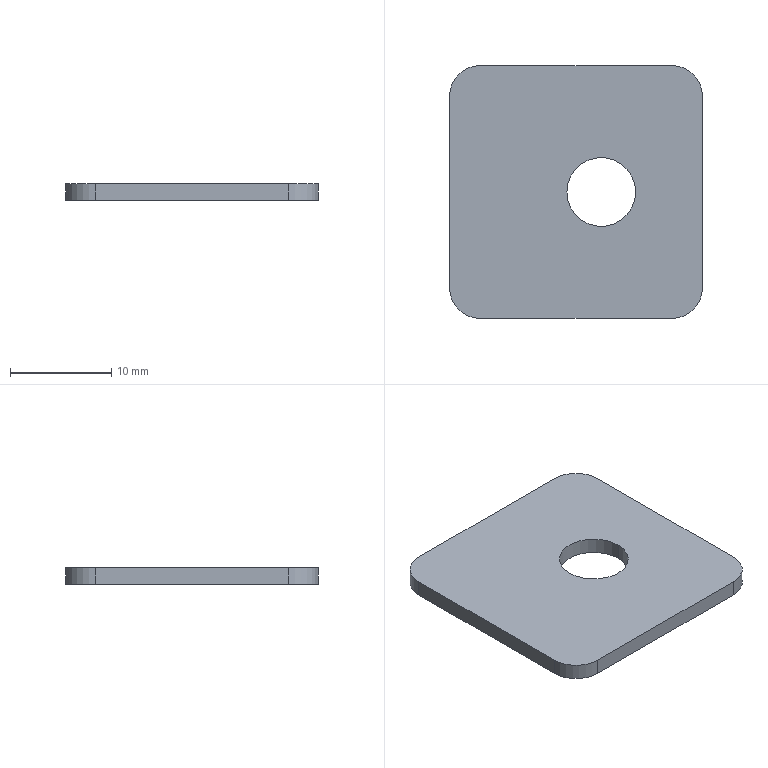Part | STEP file | J454-EBZ05-33-03-Part-1-2 | 1 solid | 12 faces | box 25 x 25 x 1.6 mm | volume 929.532 mm3 | cylinder 6 | plane 6 | commonest cylinder face diameters 6 x4 6.8 x2
STEP:
#1=CARTESIAN_POINT('',(0.,0.,0.));
#2=DIRECTION('',(0.,0.,1.));
#3=DIRECTION('',(1.,0.,0.));
#4=AXIS2_PLACEMENT_3D('',#1,#2,#3);
#5=CARTESIAN_POINT('',(11.6,12.5,0.));
#6=VERTEX_POINT('',#5);
#7=CARTESIAN_POINT('',(11.6,12.5,-1.6));
#8=VERTEX_POINT('',#7);
#9=CARTESIAN_POINT('',(11.6,12.5,0.));
#10=DIRECTION('',(0.,0.,-1.));
#11=VECTOR('',#10,1.);
#12=LINE('',#9,#11);
#13=CARTESIAN_POINT('',(15.,12.5,0.));
#14=DIRECTION('',(0.,0.,-1.));
#15=DIRECTION('',(-1.,0.,0.));
#16=AXIS2_PLACEMENT_3D('',#13,#14,#15);
#17=CYLINDRICAL_SURFACE('',#16,3.4);
#18=CARTESIAN_POINT('',(6.283,0.));
#19=DIRECTION('',(0.,1.));
#20=VECTOR('',#19,1.);
#21=LINE('',#18,#20);
#22=(GEOMETRIC_REPRESENTATION_CONTEXT(2)PARAMETRIC_REPRESENTATION_CONTEXT()REPRESENTATION_CONTEXT('',''));
#23=DEFINITIONAL_REPRESENTATION('',(#21),#22);
#24=PCURVE('',#17,#23);
#25=CARTESIAN_POINT('',(15.,12.5,0.));
#26=DIRECTION('',(0.,0.,-1.));
#27=DIRECTION('',(-1.,0.,0.));
#28=AXIS2_PLACEMENT_3D('',#25,#26,#27);
#29=CYLINDRICAL_SURFACE('',#28,3.4);
#30=CARTESIAN_POINT('',(0.,0.));
#31=DIRECTION('',(0.,1.));
#32=VECTOR('',#31,1.);
#33=LINE('',#30,#32);
#34=(GEOMETRIC_REPRESENTATION_CONTEXT(2)PARAMETRIC_REPRESENTATION_CONTEXT()REPRESENTATION_CONTEXT('',''));
#35=DEFINITIONAL_REPRESENTATION('',(#33),#34);
#36=PCURVE('',#29,#35);
#37=SURFACE_CURVE('',#12,(#24,#36),.PCURVE_S1.);
#38=EDGE_CURVE('',#6,#8,#37,.T.);
#39=ORIENTED_EDGE('',*,*,#38,.T.);
#40=CARTESIAN_POINT('',(18.4,12.5,-1.6));
#41=VERTEX_POINT('',#40);
#42=CARTESIAN_POINT('',(15.,12.5,-1.6));
#43=DIRECTION('',(0.,0.,1.));
#44=DIRECTION('',(1.,0.,0.));
#45=AXIS2_PLACEMENT_3D('',#42,#43,#44);
#46=CIRCLE('',#45,3.4);
#47=CARTESIAN_POINT('',(9.425,1.6));
#48=DIRECTION('',(-1.,0.));
#49=VECTOR('',#48,1.);
#50=LINE('',#47,#49);
#51=(GEOMETRIC_REPRESENTATION_CONTEXT(2)PARAMETRIC_REPRESENTATION_CONTEXT()REPRESENTATION_CONTEXT('',''));
#52=DEFINITIONAL_REPRESENTATION('',(#50),#51);
#53=PCURVE('',#17,#52);
#54=CARTESIAN_POINT('',(12.5,12.5,-1.6));
#55=DIRECTION('',(0.,0.,-1.));
#56=DIRECTION('',(-1.,0.,0.));
#57=AXIS2_PLACEMENT_3D('',#54,#55,#56);
#58=PLANE('',#57);
#59=CARTESIAN_POINT('',(-5.9,0.));
#60=CARTESIAN_POINT('',(-5.9,5.889));
#61=CARTESIAN_POINT('',(-0.8,2.944));
#62=CARTESIAN_POINT('',(4.3,0.));
#63=CARTESIAN_POINT('',(-0.8,-2.944));
#64=CARTESIAN_POINT('',(-5.9,-5.889));
#65=CARTESIAN_POINT('',(-5.9,0.));
#66=(BOUNDED_CURVE()B_SPLINE_CURVE(2,(#59,#60,#61,#62,#63,#64,#65),.UNSPECIFIED.,.T.,.F.)B_SPLINE_CURVE_WITH_KNOTS((1,2,2,2,2,1),(-2.094,0.,2.094,4.189,6.283,8.378),.UNSPECIFIED.)CURVE()GEOMETRIC_REPRESENTATION_ITEM()RATIONAL_B_SPLINE_CURVE((1.,0.5,1.,0.5,1.,0.5,1.))REPRESENTATION_ITEM(''));
#67=(GEOMETRIC_REPRESENTATION_CONTEXT(2)PARAMETRIC_REPRESENTATION_CONTEXT()REPRESENTATION_CONTEXT('',''));
#68=DEFINITIONAL_REPRESENTATION('',(#66),#67);
#69=PCURVE('',#58,#68);
#70=SURFACE_CURVE('',#46,(#53,#69),.PCURVE_S1.);
#71=EDGE_CURVE('',#8,#41,#70,.T.);
#72=ORIENTED_EDGE('',*,*,#71,.T.);
#73=CARTESIAN_POINT('',(18.4,12.5,0.));
#74=VERTEX_POINT('',#73);
#75=CARTESIAN_POINT('',(18.4,12.5,0.));
#76=DIRECTION('',(0.,0.,-1.));
#77=VECTOR('',#76,1.);
#78=LINE('',#75,#77);
#79=CARTESIAN_POINT('',(3.142,0.));
#80=DIRECTION('',(0.,1.));
#81=VECTOR('',#80,1.);
#82=LINE('',#79,#81);
#83=(GEOMETRIC_REPRESENTATION_CONTEXT(2)PARAMETRIC_REPRESENTATION_CONTEXT()REPRESENTATION_CONTEXT('',''));
#84=DEFINITIONAL_REPRESENTATION('',(#82),#83);
#85=PCURVE('',#17,#84);
#86=CARTESIAN_POINT('',(3.142,0.));
#87=DIRECTION('',(0.,1.));
#88=VECTOR('',#87,1.);
#89=LINE('',#86,#88);
#90=(GEOMETRIC_REPRESENTATION_CONTEXT(2)PARAMETRIC_REPRESENTATION_CONTEXT()REPRESENTATION_CONTEXT('',''));
#91=DEFINITIONAL_REPRESENTATION('',(#89),#90);
#92=PCURVE('',#29,#91);
#93=SURFACE_CURVE('',#78,(#85,#92),.PCURVE_S1.);
#94=EDGE_CURVE('',#74,#41,#93,.T.);
#95=ORIENTED_EDGE('',*,*,#94,.F.);
#96=CARTESIAN_POINT('',(15.,12.5,0.));
#97=DIRECTION('',(0.,0.,-1.));
#98=DIRECTION('',(-1.,0.,0.));
#99=AXIS2_PLACEMENT_3D('',#96,#97,#98);
#100=CIRCLE('',#99,3.4);
#101=CARTESIAN_POINT('',(0.,0.));
#102=DIRECTION('',(1.,0.));
#103=VECTOR('',#102,1.);
#104=LINE('',#101,#103);
#105=(GEOMETRIC_REPRESENTATION_CONTEXT(2)PARAMETRIC_REPRESENTATION_CONTEXT()REPRESENTATION_CONTEXT('',''));
#106=DEFINITIONAL_REPRESENTATION('',(#104),#105);
#107=PCURVE('',#17,#106);
#108=CARTESIAN_POINT('',(12.5,12.5,0.));
#109=DIRECTION('',(0.,0.,1.));
#110=DIRECTION('',(1.,0.,0.));
#111=AXIS2_PLACEMENT_3D('',#108,#109,#110);
#112=PLANE('',#111);
#113=CARTESIAN_POINT('',(-0.9,0.));
#114=CARTESIAN_POINT('',(-0.9,5.889));
#115=CARTESIAN_POINT('',(4.2,2.944));
#116=CARTESIAN_POINT('',(9.3,0.));
#117=CARTESIAN_POINT('',(4.2,-2.944));
#118=CARTESIAN_POINT('',(-0.9,-5.889));
#119=CARTESIAN_POINT('',(-0.9,0.));
#120=(BOUNDED_CURVE()B_SPLINE_CURVE(2,(#113,#114,#115,#116,#117,#118,#119),.UNSPECIFIED.,.T.,.F.)B_SPLINE_CURVE_WITH_KNOTS((1,2,2,2,2,1),(-2.094,0.,2.094,4.189,6.283,8.378),.UNSPECIFIED.)CURVE()GEOMETRIC_REPRESENTATION_ITEM()RATIONAL_B_SPLINE_CURVE((1.,0.5,1.,0.5,1.,0.5,1.))REPRESENTATION_ITEM(''));
#121=(GEOMETRIC_REPRESENTATION_CONTEXT(2)PARAMETRIC_REPRESENTATION_CONTEXT()REPRESENTATION_CONTEXT('',''));
#122=DEFINITIONAL_REPRESENTATION('',(#120),#121);
#123=PCURVE('',#112,#122);
#124=SURFACE_CURVE('',#100,(#107,#123),.PCURVE_S1.);
#125=EDGE_CURVE('',#74,#6,#124,.T.);
#126=ORIENTED_EDGE('',*,*,#125,.T.);
#127=EDGE_LOOP('',(#39,#72,#95,#126));
#128=FACE_BOUND('',#127,.F.);
#129=ADVANCED_FACE('',(#128),#17,.F.);
#130=CARTESIAN_POINT('',(15.,12.5,0.));
#131=DIRECTION('',(0.,0.,-1.));
#132=DIRECTION('',(-1.,0.,0.));
#133=AXIS2_PLACEMENT_3D('',#130,#131,#132);
#134=CIRCLE('',#133,3.4);
#135=CARTESIAN_POINT('',(-0.9,0.));
#136=CARTESIAN_POINT('',(-0.9,5.889));
#137=CARTESIAN_POINT('',(4.2,2.944));
#138=CARTESIAN_POINT('',(9.3,0.));
#139=CARTESIAN_POINT('',(4.2,-2.944));
#140=CARTESIAN_POINT('',(-0.9,-5.889));
#141=CARTESIAN_POINT('',(-0.9,0.));
#142=(BOUNDED_CURVE()B_SPLINE_CURVE(2,(#135,#136,#137,#138,#139,#140,#141),.UNSPECIFIED.,.T.,.F.)B_SPLINE_CURVE_WITH_KNOTS((1,2,2,2,2,1),(-2.094,0.,2.094,4.189,6.283,8.378),.UNSPECIFIED.)CURVE()GEOMETRIC_REPRESENTATION_ITEM()RATIONAL_B_SPLINE_CURVE((1.,0.5,1.,0.5,1.,0.5,1.))REPRESENTATION_ITEM(''));
#143=(GEOMETRIC_REPRESENTATION_CONTEXT(2)PARAMETRIC_REPRESENTATION_CONTEXT()REPRESENTATION_CONTEXT('',''));
#144=DEFINITIONAL_REPRESENTATION('',(#142),#143);
#145=PCURVE('',#112,#144);
#146=CARTESIAN_POINT('',(0.,0.));
#147=DIRECTION('',(1.,0.));
#148=VECTOR('',#147,1.);
#149=LINE('',#146,#148);
#150=(GEOMETRIC_REPRESENTATION_CONTEXT(2)PARAMETRIC_REPRESENTATION_CONTEXT()REPRESENTATION_CONTEXT('',''));
#151=DEFINITIONAL_REPRESENTATION('',(#149),#150);
#152=PCURVE('',#29,#151);
#153=SURFACE_CURVE('',#134,(#145,#152),.PCURVE_S1.);
#154=EDGE_CURVE('',#6,#74,#153,.T.);
#155=ORIENTED_EDGE('',*,*,#154,.T.);
#156=ORIENTED_EDGE('',*,*,#125,.T.);
#157=EDGE_LOOP('',(#155,#156));
#158=FACE_BOUND('',#157,.T.);
#159=CARTESIAN_POINT('',(25.,22.,0.));
#160=VERTEX_POINT('',#159);
#161=CARTESIAN_POINT('',(25.,3.,0.));
#162=VERTEX_POINT('',#161);
#163=CARTESIAN_POINT('',(25.,12.5,0.));
#164=DIRECTION('',(0.,-1.,0.));
#165=VECTOR('',#164,1.);
#166=LINE('',#163,#165);
#167=CARTESIAN_POINT('',(12.5,0.));
#168=DIRECTION('',(0.,-1.));
#169=VECTOR('',#168,1.);
#170=LINE('',#167,#169);
#171=(GEOMETRIC_REPRESENTATION_CONTEXT(2)PARAMETRIC_REPRESENTATION_CONTEXT()REPRESENTATION_CONTEXT('',''));
#172=DEFINITIONAL_REPRESENTATION('',(#170),#171);
#173=PCURVE('',#112,#172);
#174=CARTESIAN_POINT('',(25.,12.5,-1.6));
#175=DIRECTION('',(1.,0.,0.));
#176=DIRECTION('',(0.,0.,-1.));
#177=AXIS2_PLACEMENT_3D('',#174,#175,#176);
#178=PLANE('',#177);
#179=CARTESIAN_POINT('',(-1.6,0.));
#180=DIRECTION('',(0.,-1.));
#181=VECTOR('',#180,1.);
#182=LINE('',#179,#181);
#183=(GEOMETRIC_REPRESENTATION_CONTEXT(2)PARAMETRIC_REPRESENTATION_CONTEXT()REPRESENTATION_CONTEXT('',''));
#184=DEFINITIONAL_REPRESENTATION('',(#182),#183);
#185=PCURVE('',#178,#184);
#186=SURFACE_CURVE('',#166,(#173,#185),.PCURVE_S1.);
#187=EDGE_CURVE('',#160,#162,#186,.T.);
#188=ORIENTED_EDGE('',*,*,#187,.F.);
#189=CARTESIAN_POINT('',(22.,25.,0.));
#190=VERTEX_POINT('',#189);
#191=CARTESIAN_POINT('',(22.,22.,0.));
#192=DIRECTION('',(0.,0.,1.));
#193=DIRECTION('',(1.,0.,0.));
#194=AXIS2_PLACEMENT_3D('',#191,#192,#193);
#195=CIRCLE('',#194,3.);
#196=CARTESIAN_POINT('',(9.5,9.5));
#197=DIRECTION('',(1.,0.));
#198=AXIS2_PLACEMENT_2D('',#196,#197);
#199=CIRCLE('',#198,3.);
#200=(GEOMETRIC_REPRESENTATION_CONTEXT(2)PARAMETRIC_REPRESENTATION_CONTEXT()REPRESENTATION_CONTEXT('',''));
#201=DEFINITIONAL_REPRESENTATION('',(#199),#200);
#202=PCURVE('',#112,#201);
#203=CARTESIAN_POINT('',(22.,22.,-1.6));
#204=DIRECTION('',(0.,0.,1.));
#205=DIRECTION('',(1.,0.,0.));
#206=AXIS2_PLACEMENT_3D('',#203,#204,#205);
#207=CYLINDRICAL_SURFACE('',#206,3.);
#208=CARTESIAN_POINT('',(0.,1.6));
#209=DIRECTION('',(1.,0.));
#210=VECTOR('',#209,1.);
#211=LINE('',#208,#210);
#212=(GEOMETRIC_REPRESENTATION_CONTEXT(2)PARAMETRIC_REPRESENTATION_CONTEXT()REPRESENTATION_CONTEXT('',''));
#213=DEFINITIONAL_REPRESENTATION('',(#211),#212);
#214=PCURVE('',#207,#213);
#215=SURFACE_CURVE('',#195,(#202,#214),.PCURVE_S1.);
#216=EDGE_CURVE('',#160,#190,#215,.T.);
#217=ORIENTED_EDGE('',*,*,#216,.T.);
#218=CARTESIAN_POINT('',(3.,25.,0.));
#219=VERTEX_POINT('',#218);
#220=CARTESIAN_POINT('',(12.5,25.,0.));
#221=DIRECTION('',(1.,0.,0.));
#222=VECTOR('',#221,1.);
#223=LINE('',#220,#222);
#224=CARTESIAN_POINT('',(0.,12.5));
#225=DIRECTION('',(1.,0.));
#226=VECTOR('',#225,1.);
#227=LINE('',#224,#226);
#228=(GEOMETRIC_REPRESENTATION_CONTEXT(2)PARAMETRIC_REPRESENTATION_CONTEXT()REPRESENTATION_CONTEXT('',''));
#229=DEFINITIONAL_REPRESENTATION('',(#227),#228);
#230=PCURVE('',#112,#229);
#231=CARTESIAN_POINT('',(12.5,25.,-1.6));
#232=DIRECTION('',(0.,1.,0.));
#233=DIRECTION('',(0.,0.,1.));
#234=AXIS2_PLACEMENT_3D('',#231,#232,#233);
#235=PLANE('',#234);
#236=CARTESIAN_POINT('',(1.6,0.));
#237=DIRECTION('',(0.,1.));
#238=VECTOR('',#237,1.);
#239=LINE('',#236,#238);
#240=(GEOMETRIC_REPRESENTATION_CONTEXT(2)PARAMETRIC_REPRESENTATION_CONTEXT()REPRESENTATION_CONTEXT('',''));
#241=DEFINITIONAL_REPRESENTATION('',(#239),#240);
#242=PCURVE('',#235,#241);
#243=SURFACE_CURVE('',#223,(#230,#242),.PCURVE_S1.);
#244=EDGE_CURVE('',#219,#190,#243,.T.);
#245=ORIENTED_EDGE('',*,*,#244,.F.);
#246=CARTESIAN_POINT('',(0.,22.,0.));
#247=VERTEX_POINT('',#246);
#248=CARTESIAN_POINT('',(3.,22.,0.));
#249=DIRECTION('',(0.,0.,1.));
#250=DIRECTION('',(1.,0.,0.));
#251=AXIS2_PLACEMENT_3D('',#248,#249,#250);
#252=CIRCLE('',#251,3.);
#253=CARTESIAN_POINT('',(-9.5,9.5));
#254=DIRECTION('',(1.,0.));
#255=AXIS2_PLACEMENT_2D('',#253,#254);
#256=CIRCLE('',#255,3.);
#257=(GEOMETRIC_REPRESENTATION_CONTEXT(2)PARAMETRIC_REPRESENTATION_CONTEXT()REPRESENTATION_CONTEXT('',''));
#258=DEFINITIONAL_REPRESENTATION('',(#256),#257);
#259=PCURVE('',#112,#258);
#260=CARTESIAN_POINT('',(3.,22.,-1.6));
#261=DIRECTION('',(0.,0.,1.));
#262=DIRECTION('',(1.,0.,0.));
#263=AXIS2_PLACEMENT_3D('',#260,#261,#262);
#264=CYLINDRICAL_SURFACE('',#263,3.);
#265=CARTESIAN_POINT('',(0.,1.6));
#266=DIRECTION('',(1.,0.));
#267=VECTOR('',#266,1.);
#268=LINE('',#265,#267);
#269=(GEOMETRIC_REPRESENTATION_CONTEXT(2)PARAMETRIC_REPRESENTATION_CONTEXT()REPRESENTATION_CONTEXT('',''));
#270=DEFINITIONAL_REPRESENTATION('',(#268),#269);
#271=PCURVE('',#264,#270);
#272=SURFACE_CURVE('',#252,(#259,#271),.PCURVE_S1.);
#273=EDGE_CURVE('',#219,#247,#272,.T.);
#274=ORIENTED_EDGE('',*,*,#273,.T.);
#275=CARTESIAN_POINT('',(0.,3.,0.));
#276=VERTEX_POINT('',#275);
#277=CARTESIAN_POINT('',(0.,12.5,0.));
#278=DIRECTION('',(0.,1.,0.));
#279=VECTOR('',#278,1.);
#280=LINE('',#277,#279);
#281=CARTESIAN_POINT('',(-12.5,0.));
#282=DIRECTION('',(0.,1.));
#283=VECTOR('',#282,1.);
#284=LINE('',#281,#283);
#285=(GEOMETRIC_REPRESENTATION_CONTEXT(2)PARAMETRIC_REPRESENTATION_CONTEXT()REPRESENTATION_CONTEXT('',''));
#286=DEFINITIONAL_REPRESENTATION('',(#284),#285);
#287=PCURVE('',#112,#286);
#288=CARTESIAN_POINT('',(0.,12.5,-1.6));
#289=DIRECTION('',(-1.,0.,0.));
#290=DIRECTION('',(0.,0.,1.));
#291=AXIS2_PLACEMENT_3D('',#288,#289,#290);
#292=PLANE('',#291);
#293=CARTESIAN_POINT('',(1.6,0.));
#294=DIRECTION('',(0.,1.));
#295=VECTOR('',#294,1.);
#296=LINE('',#293,#295);
#297=(GEOMETRIC_REPRESENTATION_CONTEXT(2)PARAMETRIC_REPRESENTATION_CONTEXT()REPRESENTATION_CONTEXT('',''));
#298=DEFINITIONAL_REPRESENTATION('',(#296),#297);
#299=PCURVE('',#292,#298);
#300=SURFACE_CURVE('',#280,(#287,#299),.PCURVE_S1.);
#301=EDGE_CURVE('',#276,#247,#300,.T.);
#302=ORIENTED_EDGE('',*,*,#301,.F.);
#303=CARTESIAN_POINT('',(3.,0.,0.));
#304=VERTEX_POINT('',#303);
#305=CARTESIAN_POINT('',(3.,3.,0.));
#306=DIRECTION('',(0.,0.,1.));
#307=DIRECTION('',(1.,0.,0.));
#308=AXIS2_PLACEMENT_3D('',#305,#306,#307);
#309=CIRCLE('',#308,3.);
#310=CARTESIAN_POINT('',(-9.5,-9.5));
#311=DIRECTION('',(1.,0.));
#312=AXIS2_PLACEMENT_2D('',#310,#311);
#313=CIRCLE('',#312,3.);
#314=(GEOMETRIC_REPRESENTATION_CONTEXT(2)PARAMETRIC_REPRESENTATION_CONTEXT()REPRESENTATION_CONTEXT('',''));
#315=DEFINITIONAL_REPRESENTATION('',(#313),#314);
#316=PCURVE('',#112,#315);
#317=CARTESIAN_POINT('',(3.,3.,-1.6));
#318=DIRECTION('',(0.,0.,1.));
#319=DIRECTION('',(1.,0.,0.));
#320=AXIS2_PLACEMENT_3D('',#317,#318,#319);
#321=CYLINDRICAL_SURFACE('',#320,3.);
#322=CARTESIAN_POINT('',(0.,1.6));
#323=DIRECTION('',(1.,0.));
#324=VECTOR('',#323,1.);
#325=LINE('',#322,#324);
#326=(GEOMETRIC_REPRESENTATION_CONTEXT(2)PARAMETRIC_REPRESENTATION_CONTEXT()REPRESENTATION_CONTEXT('',''));
#327=DEFINITIONAL_REPRESENTATION('',(#325),#326);
#328=PCURVE('',#321,#327);
#329=SURFACE_CURVE('',#309,(#316,#328),.PCURVE_S1.);
#330=EDGE_CURVE('',#276,#304,#329,.T.);
#331=ORIENTED_EDGE('',*,*,#330,.T.);
#332=CARTESIAN_POINT('',(22.,0.,0.));
#333=VERTEX_POINT('',#332);
#334=CARTESIAN_POINT('',(12.5,0.,0.));
#335=DIRECTION('',(-1.,0.,0.));
#336=VECTOR('',#335,1.);
#337=LINE('',#334,#336);
#338=CARTESIAN_POINT('',(0.,-12.5));
#339=DIRECTION('',(-1.,0.));
#340=VECTOR('',#339,1.);
#341=LINE('',#338,#340);
#342=(GEOMETRIC_REPRESENTATION_CONTEXT(2)PARAMETRIC_REPRESENTATION_CONTEXT()REPRESENTATION_CONTEXT('',''));
#343=DEFINITIONAL_REPRESENTATION('',(#341),#342);
#344=PCURVE('',#112,#343);
#345=CARTESIAN_POINT('',(12.5,0.,-1.6));
#346=DIRECTION('',(0.,-1.,0.));
#347=DIRECTION('',(0.,0.,-1.));
#348=AXIS2_PLACEMENT_3D('',#345,#346,#347);
#349=PLANE('',#348);
#350=CARTESIAN_POINT('',(-1.6,0.));
#351=DIRECTION('',(0.,-1.));
#352=VECTOR('',#351,1.);
#353=LINE('',#350,#352);
#354=(GEOMETRIC_REPRESENTATION_CONTEXT(2)PARAMETRIC_REPRESENTATION_CONTEXT()REPRESENTATION_CONTEXT('',''));
#355=DEFINITIONAL_REPRESENTATION('',(#353),#354);
#356=PCURVE('',#349,#355);
#357=SURFACE_CURVE('',#337,(#344,#356),.PCURVE_S1.);
#358=EDGE_CURVE('',#333,#304,#357,.T.);
#359=ORIENTED_EDGE('',*,*,#358,.F.);
#360=CARTESIAN_POINT('',(22.,3.,0.));
#361=DIRECTION('',(0.,0.,1.));
#362=DIRECTION('',(1.,0.,0.));
#363=AXIS2_PLACEMENT_3D('',#360,#361,#362);
#364=CIRCLE('',#363,3.);
#365=CARTESIAN_POINT('',(9.5,-9.5));
#366=DIRECTION('',(1.,0.));
#367=AXIS2_PLACEMENT_2D('',#365,#366);
#368=CIRCLE('',#367,3.);
#369=(GEOMETRIC_REPRESENTATION_CONTEXT(2)PARAMETRIC_REPRESENTATION_CONTEXT()REPRESENTATION_CONTEXT('',''));
#370=DEFINITIONAL_REPRESENTATION('',(#368),#369);
#371=PCURVE('',#112,#370);
#372=CARTESIAN_POINT('',(22.,3.,-1.6));
#373=DIRECTION('',(0.,0.,1.));
#374=DIRECTION('',(1.,0.,0.));
#375=AXIS2_PLACEMENT_3D('',#372,#373,#374);
#376=CYLINDRICAL_SURFACE('',#375,3.);
#377=CARTESIAN_POINT('',(0.,1.6));
#378=DIRECTION('',(1.,0.));
#379=VECTOR('',#378,1.);
#380=LINE('',#377,#379);
#381=(GEOMETRIC_REPRESENTATION_CONTEXT(2)PARAMETRIC_REPRESENTATION_CONTEXT()REPRESENTATION_CONTEXT('',''));
#382=DEFINITIONAL_REPRESENTATION('',(#380),#381);
#383=PCURVE('',#376,#382);
#384=SURFACE_CURVE('',#364,(#371,#383),.PCURVE_S1.);
#385=EDGE_CURVE('',#333,#162,#384,.T.);
#386=ORIENTED_EDGE('',*,*,#385,.T.);
#387=EDGE_LOOP('',(#188,#217,#245,#274,#302,#331,#359,#386));
#388=FACE_BOUND('',#387,.T.);
#389=ADVANCED_FACE('',(#158,#388),#112,.T.);
#390=CARTESIAN_POINT('',(3.,0.,-1.6));
#391=VERTEX_POINT('',#390);
#392=CARTESIAN_POINT('',(22.,0.,-1.6));
#393=VERTEX_POINT('',#392);
#394=CARTESIAN_POINT('',(12.5,0.,-1.6));
#395=DIRECTION('',(1.,0.,0.));
#396=VECTOR('',#395,1.);
#397=LINE('',#394,#396);
#398=CARTESIAN_POINT('',(0.,0.));
#399=DIRECTION('',(0.,1.));
#400=VECTOR('',#399,1.);
#401=LINE('',#398,#400);
#402=(GEOMETRIC_REPRESENTATION_CONTEXT(2)PARAMETRIC_REPRESENTATION_CONTEXT()REPRESENTATION_CONTEXT('',''));
#403=DEFINITIONAL_REPRESENTATION('',(#401),#402);
#404=PCURVE('',#349,#403);
#405=CARTESIAN_POINT('',(0.,-12.5));
#406=DIRECTION('',(-1.,0.));
#407=VECTOR('',#406,1.);
#408=LINE('',#405,#407);
#409=(GEOMETRIC_REPRESENTATION_CONTEXT(2)PARAMETRIC_REPRESENTATION_CONTEXT()REPRESENTATION_CONTEXT('',''));
#410=DEFINITIONAL_REPRESENTATION('',(#408),#409);
#411=PCURVE('',#58,#410);
#412=SURFACE_CURVE('',#397,(#404,#411),.PCURVE_S1.);
#413=EDGE_CURVE('',#391,#393,#412,.T.);
#414=ORIENTED_EDGE('',*,*,#413,.T.);
#415=CARTESIAN_POINT('',(22.,0.,-1.6));
#416=DIRECTION('',(0.,0.,1.));
#417=VECTOR('',#416,1.);
#418=LINE('',#415,#417);
#419=CARTESIAN_POINT('',(0.,9.5));
#420=DIRECTION('',(-1.,0.));
#421=VECTOR('',#420,1.);
#422=LINE('',#419,#421);
#423=(GEOMETRIC_REPRESENTATION_CONTEXT(2)PARAMETRIC_REPRESENTATION_CONTEXT()REPRESENTATION_CONTEXT('',''));
#424=DEFINITIONAL_REPRESENTATION('',(#422),#423);
#425=PCURVE('',#349,#424);
#426=CARTESIAN_POINT('',(4.712,0.));
#427=DIRECTION('',(0.,1.));
#428=VECTOR('',#427,1.);
#429=LINE('',#426,#428);
#430=(GEOMETRIC_REPRESENTATION_CONTEXT(2)PARAMETRIC_REPRESENTATION_CONTEXT()REPRESENTATION_CONTEXT('',''));
#431=DEFINITIONAL_REPRESENTATION('',(#429),#430);
#432=PCURVE('',#376,#431);
#433=SURFACE_CURVE('',#418,(#425,#432),.PCURVE_S1.);
#434=EDGE_CURVE('',#393,#333,#433,.T.);
#435=ORIENTED_EDGE('',*,*,#434,.T.);
#436=ORIENTED_EDGE('',*,*,#358,.T.);
#437=CARTESIAN_POINT('',(3.,0.,-1.6));
#438=DIRECTION('',(0.,0.,-1.));
#439=VECTOR('',#438,1.);
#440=LINE('',#437,#439);
#441=CARTESIAN_POINT('',(0.,-9.5));
#442=DIRECTION('',(1.,0.));
#443=VECTOR('',#442,1.);
#444=LINE('',#441,#443);
#445=(GEOMETRIC_REPRESENTATION_CONTEXT(2)PARAMETRIC_REPRESENTATION_CONTEXT()REPRESENTATION_CONTEXT('',''));
#446=DEFINITIONAL_REPRESENTATION('',(#444),#445);
#447=PCURVE('',#349,#446);
#448=CARTESIAN_POINT('',(4.712,0.));
#449=DIRECTION('',(0.,-1.));
#450=VECTOR('',#449,1.);
#451=LINE('',#448,#450);
#452=(GEOMETRIC_REPRESENTATION_CONTEXT(2)PARAMETRIC_REPRESENTATION_CONTEXT()REPRESENTATION_CONTEXT('',''));
#453=DEFINITIONAL_REPRESENTATION('',(#451),#452);
#454=PCURVE('',#321,#453);
#455=SURFACE_CURVE('',#440,(#447,#454),.PCURVE_S1.);
#456=EDGE_CURVE('',#304,#391,#455,.T.);
#457=ORIENTED_EDGE('',*,*,#456,.T.);
#458=EDGE_LOOP('',(#414,#435,#436,#457));
#459=FACE_BOUND('',#458,.T.);
#460=ADVANCED_FACE('',(#459),#349,.T.);
#461=CARTESIAN_POINT('',(0.,22.,-1.6));
#462=VERTEX_POINT('',#461);
#463=CARTESIAN_POINT('',(0.,3.,-1.6));
#464=VERTEX_POINT('',#463);
#465=CARTESIAN_POINT('',(0.,12.5,-1.6));
#466=DIRECTION('',(0.,-1.,0.));
#467=VECTOR('',#466,1.);
#468=LINE('',#465,#467);
#469=CARTESIAN_POINT('',(0.,0.));
#470=DIRECTION('',(0.,-1.));
#471=VECTOR('',#470,1.);
#472=LINE('',#469,#471);
#473=(GEOMETRIC_REPRESENTATION_CONTEXT(2)PARAMETRIC_REPRESENTATION_CONTEXT()REPRESENTATION_CONTEXT('',''));
#474=DEFINITIONAL_REPRESENTATION('',(#472),#473);
#475=PCURVE('',#292,#474);
#476=CARTESIAN_POINT('',(12.5,0.));
#477=DIRECTION('',(0.,-1.));
#478=VECTOR('',#477,1.);
#479=LINE('',#476,#478);
#480=(GEOMETRIC_REPRESENTATION_CONTEXT(2)PARAMETRIC_REPRESENTATION_CONTEXT()REPRESENTATION_CONTEXT('',''));
#481=DEFINITIONAL_REPRESENTATION('',(#479),#480);
#482=PCURVE('',#58,#481);
#483=SURFACE_CURVE('',#468,(#475,#482),.PCURVE_S1.);
#484=EDGE_CURVE('',#462,#464,#483,.T.);
#485=ORIENTED_EDGE('',*,*,#484,.T.);
#486=CARTESIAN_POINT('',(0.,3.,-1.6));
#487=DIRECTION('',(0.,0.,1.));
#488=VECTOR('',#487,1.);
#489=LINE('',#486,#488);
#490=CARTESIAN_POINT('',(0.,-9.5));
#491=DIRECTION('',(1.,0.));
#492=VECTOR('',#491,1.);
#493=LINE('',#490,#492);
#494=(GEOMETRIC_REPRESENTATION_CONTEXT(2)PARAMETRIC_REPRESENTATION_CONTEXT()REPRESENTATION_CONTEXT('',''));
#495=DEFINITIONAL_REPRESENTATION('',(#493),#494);
#496=PCURVE('',#292,#495);
#497=CARTESIAN_POINT('',(3.142,0.));
#498=DIRECTION('',(0.,1.));
#499=VECTOR('',#498,1.);
#500=LINE('',#497,#499);
#501=(GEOMETRIC_REPRESENTATION_CONTEXT(2)PARAMETRIC_REPRESENTATION_CONTEXT()REPRESENTATION_CONTEXT('',''));
#502=DEFINITIONAL_REPRESENTATION('',(#500),#501);
#503=PCURVE('',#321,#502);
#504=SURFACE_CURVE('',#489,(#496,#503),.PCURVE_S1.);
#505=EDGE_CURVE('',#464,#276,#504,.T.);
#506=ORIENTED_EDGE('',*,*,#505,.T.);
#507=ORIENTED_EDGE('',*,*,#301,.T.);
#508=CARTESIAN_POINT('',(0.,22.,-1.6));
#509=DIRECTION('',(0.,0.,-1.));
#510=VECTOR('',#509,1.);
#511=LINE('',#508,#510);
#512=CARTESIAN_POINT('',(0.,9.5));
#513=DIRECTION('',(-1.,0.));
#514=VECTOR('',#513,1.);
#515=LINE('',#512,#514);
#516=(GEOMETRIC_REPRESENTATION_CONTEXT(2)PARAMETRIC_REPRESENTATION_CONTEXT()REPRESENTATION_CONTEXT('',''));
#517=DEFINITIONAL_REPRESENTATION('',(#515),#516);
#518=PCURVE('',#292,#517);
#519=CARTESIAN_POINT('',(3.142,0.));
#520=DIRECTION('',(0.,-1.));
#521=VECTOR('',#520,1.);
#522=LINE('',#519,#521);
#523=(GEOMETRIC_REPRESENTATION_CONTEXT(2)PARAMETRIC_REPRESENTATION_CONTEXT()REPRESENTATION_CONTEXT('',''));
#524=DEFINITIONAL_REPRESENTATION('',(#522),#523);
#525=PCURVE('',#264,#524);
#526=SURFACE_CURVE('',#511,(#518,#525),.PCURVE_S1.);
#527=EDGE_CURVE('',#247,#462,#526,.T.);
#528=ORIENTED_EDGE('',*,*,#527,.T.);
#529=EDGE_LOOP('',(#485,#506,#507,#528));
#530=FACE_BOUND('',#529,.T.);
#531=ADVANCED_FACE('',(#530),#292,.T.);
#532=ORIENTED_EDGE('',*,*,#244,.T.);
#533=CARTESIAN_POINT('',(22.,25.,-1.6));
#534=VERTEX_POINT('',#533);
#535=CARTESIAN_POINT('',(22.,25.,-1.6));
#536=DIRECTION('',(0.,0.,-1.));
#537=VECTOR('',#536,1.);
#538=LINE('',#535,#537);
#539=CARTESIAN_POINT('',(0.,9.5));
#540=DIRECTION('',(-1.,0.));
#541=VECTOR('',#540,1.);
#542=LINE('',#539,#541);
#543=(GEOMETRIC_REPRESENTATION_CONTEXT(2)PARAMETRIC_REPRESENTATION_CONTEXT()REPRESENTATION_CONTEXT('',''));
#544=DEFINITIONAL_REPRESENTATION('',(#542),#543);
#545=PCURVE('',#235,#544);
#546=CARTESIAN_POINT('',(1.571,0.));
#547=DIRECTION('',(0.,-1.));
#548=VECTOR('',#547,1.);
#549=LINE('',#546,#548);
#550=(GEOMETRIC_REPRESENTATION_CONTEXT(2)PARAMETRIC_REPRESENTATION_CONTEXT()REPRESENTATION_CONTEXT('',''));
#551=DEFINITIONAL_REPRESENTATION('',(#549),#550);
#552=PCURVE('',#207,#551);
#553=SURFACE_CURVE('',#538,(#545,#552),.PCURVE_S1.);
#554=EDGE_CURVE('',#190,#534,#553,.T.);
#555=ORIENTED_EDGE('',*,*,#554,.T.);
#556=CARTESIAN_POINT('',(3.,25.,-1.6));
#557=VERTEX_POINT('',#556);
#558=CARTESIAN_POINT('',(12.5,25.,-1.6));
#559=DIRECTION('',(-1.,0.,0.));
#560=VECTOR('',#559,1.);
#561=LINE('',#558,#560);
#562=CARTESIAN_POINT('',(0.,0.));
#563=DIRECTION('',(0.,-1.));
#564=VECTOR('',#563,1.);
#565=LINE('',#562,#564);
#566=(GEOMETRIC_REPRESENTATION_CONTEXT(2)PARAMETRIC_REPRESENTATION_CONTEXT()REPRESENTATION_CONTEXT('',''));
#567=DEFINITIONAL_REPRESENTATION('',(#565),#566);
#568=PCURVE('',#235,#567);
#569=CARTESIAN_POINT('',(0.,12.5));
#570=DIRECTION('',(1.,0.));
#571=VECTOR('',#570,1.);
#572=LINE('',#569,#571);
#573=(GEOMETRIC_REPRESENTATION_CONTEXT(2)PARAMETRIC_REPRESENTATION_CONTEXT()REPRESENTATION_CONTEXT('',''));
#574=DEFINITIONAL_REPRESENTATION('',(#572),#573);
#575=PCURVE('',#58,#574);
#576=SURFACE_CURVE('',#561,(#568,#575),.PCURVE_S1.);
#577=EDGE_CURVE('',#534,#557,#576,.T.);
#578=ORIENTED_EDGE('',*,*,#577,.T.);
#579=CARTESIAN_POINT('',(3.,25.,-1.6));
#580=DIRECTION('',(0.,0.,1.));
#581=VECTOR('',#580,1.);
#582=LINE('',#579,#581);
#583=CARTESIAN_POINT('',(0.,-9.5));
#584=DIRECTION('',(1.,0.));
#585=VECTOR('',#584,1.);
#586=LINE('',#583,#585);
#587=(GEOMETRIC_REPRESENTATION_CONTEXT(2)PARAMETRIC_REPRESENTATION_CONTEXT()REPRESENTATION_CONTEXT('',''));
#588=DEFINITIONAL_REPRESENTATION('',(#586),#587);
#589=PCURVE('',#235,#588);
#590=CARTESIAN_POINT('',(1.571,0.));
#591=DIRECTION('',(0.,1.));
#592=VECTOR('',#591,1.);
#593=LINE('',#590,#592);
#594=(GEOMETRIC_REPRESENTATION_CONTEXT(2)PARAMETRIC_REPRESENTATION_CONTEXT()REPRESENTATION_CONTEXT('',''));
#595=DEFINITIONAL_REPRESENTATION('',(#593),#594);
#596=PCURVE('',#264,#595);
#597=SURFACE_CURVE('',#582,(#589,#596),.PCURVE_S1.);
#598=EDGE_CURVE('',#557,#219,#597,.T.);
#599=ORIENTED_EDGE('',*,*,#598,.T.);
#600=EDGE_LOOP('',(#532,#555,#578,#599));
#601=FACE_BOUND('',#600,.T.);
#602=ADVANCED_FACE('',(#601),#235,.T.);
#603=ORIENTED_EDGE('',*,*,#71,.T.);
#604=CARTESIAN_POINT('',(15.,12.5,-1.6));
#605=DIRECTION('',(0.,0.,1.));
#606=DIRECTION('',(1.,0.,0.));
#607=AXIS2_PLACEMENT_3D('',#604,#605,#606);
#608=CIRCLE('',#607,3.4);
#609=CARTESIAN_POINT('',(-5.9,0.));
#610=CARTESIAN_POINT('',(-5.9,5.889));
#611=CARTESIAN_POINT('',(-0.8,2.944));
#612=CARTESIAN_POINT('',(4.3,0.));
#613=CARTESIAN_POINT('',(-0.8,-2.944));
#614=CARTESIAN_POINT('',(-5.9,-5.889));
#615=CARTESIAN_POINT('',(-5.9,0.));
#616=(BOUNDED_CURVE()B_SPLINE_CURVE(2,(#609,#610,#611,#612,#613,#614,#615),.UNSPECIFIED.,.T.,.F.)B_SPLINE_CURVE_WITH_KNOTS((1,2,2,2,2,1),(-2.094,0.,2.094,4.189,6.283,8.378),.UNSPECIFIED.)CURVE()GEOMETRIC_REPRESENTATION_ITEM()RATIONAL_B_SPLINE_CURVE((1.,0.5,1.,0.5,1.,0.5,1.))REPRESENTATION_ITEM(''));
#617=(GEOMETRIC_REPRESENTATION_CONTEXT(2)PARAMETRIC_REPRESENTATION_CONTEXT()REPRESENTATION_CONTEXT('',''));
#618=DEFINITIONAL_REPRESENTATION('',(#616),#617);
#619=PCURVE('',#58,#618);
#620=CARTESIAN_POINT('',(3.142,1.6));
#621=DIRECTION('',(-1.,0.));
#622=VECTOR('',#621,1.);
#623=LINE('',#620,#622);
#624=(GEOMETRIC_REPRESENTATION_CONTEXT(2)PARAMETRIC_REPRESENTATION_CONTEXT()REPRESENTATION_CONTEXT('',''));
#625=DEFINITIONAL_REPRESENTATION('',(#623),#624);
#626=PCURVE('',#29,#625);
#627=SURFACE_CURVE('',#608,(#619,#626),.PCURVE_S1.);
#628=EDGE_CURVE('',#41,#8,#627,.T.);
#629=ORIENTED_EDGE('',*,*,#628,.T.);
#630=EDGE_LOOP('',(#603,#629));
#631=FACE_BOUND('',#630,.T.);
#632=ORIENTED_EDGE('',*,*,#577,.F.);
#633=CARTESIAN_POINT('',(25.,22.,-1.6));
#634=VERTEX_POINT('',#633);
#635=CARTESIAN_POINT('',(22.,22.,-1.6));
#636=DIRECTION('',(0.,0.,-1.));
#637=DIRECTION('',(-1.,0.,0.));
#638=AXIS2_PLACEMENT_3D('',#635,#636,#637);
#639=CIRCLE('',#638,3.);
#640=CARTESIAN_POINT('',(-9.5,9.5));
#641=DIRECTION('',(1.,0.));
#642=AXIS2_PLACEMENT_2D('',#640,#641);
#643=CIRCLE('',#642,3.);
#644=(GEOMETRIC_REPRESENTATION_CONTEXT(2)PARAMETRIC_REPRESENTATION_CONTEXT()REPRESENTATION_CONTEXT('',''));
#645=DEFINITIONAL_REPRESENTATION('',(#643),#644);
#646=PCURVE('',#58,#645);
#647=CARTESIAN_POINT('',(3.142,0.));
#648=DIRECTION('',(-1.,0.));
#649=VECTOR('',#648,1.);
#650=LINE('',#647,#649);
#651=(GEOMETRIC_REPRESENTATION_CONTEXT(2)PARAMETRIC_REPRESENTATION_CONTEXT()REPRESENTATION_CONTEXT('',''));
#652=DEFINITIONAL_REPRESENTATION('',(#650),#651);
#653=PCURVE('',#207,#652);
#654=SURFACE_CURVE('',#639,(#646,#653),.PCURVE_S1.);
#655=EDGE_CURVE('',#534,#634,#654,.T.);
#656=ORIENTED_EDGE('',*,*,#655,.T.);
#657=CARTESIAN_POINT('',(25.,3.,-1.6));
#658=VERTEX_POINT('',#657);
#659=CARTESIAN_POINT('',(25.,12.5,-1.6));
#660=DIRECTION('',(0.,1.,0.));
#661=VECTOR('',#660,1.);
#662=LINE('',#659,#661);
#663=CARTESIAN_POINT('',(-12.5,0.));
#664=DIRECTION('',(0.,1.));
#665=VECTOR('',#664,1.);
#666=LINE('',#663,#665);
#667=(GEOMETRIC_REPRESENTATION_CONTEXT(2)PARAMETRIC_REPRESENTATION_CONTEXT()REPRESENTATION_CONTEXT('',''));
#668=DEFINITIONAL_REPRESENTATION('',(#666),#667);
#669=PCURVE('',#58,#668);
#670=CARTESIAN_POINT('',(0.,0.));
#671=DIRECTION('',(0.,1.));
#672=VECTOR('',#671,1.);
#673=LINE('',#670,#672);
#674=(GEOMETRIC_REPRESENTATION_CONTEXT(2)PARAMETRIC_REPRESENTATION_CONTEXT()REPRESENTATION_CONTEXT('',''));
#675=DEFINITIONAL_REPRESENTATION('',(#673),#674);
#676=PCURVE('',#178,#675);
#677=SURFACE_CURVE('',#662,(#669,#676),.PCURVE_S1.);
#678=EDGE_CURVE('',#658,#634,#677,.T.);
#679=ORIENTED_EDGE('',*,*,#678,.F.);
#680=CARTESIAN_POINT('',(22.,3.,-1.6));
#681=DIRECTION('',(0.,0.,-1.));
#682=DIRECTION('',(-1.,0.,0.));
#683=AXIS2_PLACEMENT_3D('',#680,#681,#682);
#684=CIRCLE('',#683,3.);
#685=CARTESIAN_POINT('',(-9.5,-9.5));
#686=DIRECTION('',(1.,0.));
#687=AXIS2_PLACEMENT_2D('',#685,#686);
#688=CIRCLE('',#687,3.);
#689=(GEOMETRIC_REPRESENTATION_CONTEXT(2)PARAMETRIC_REPRESENTATION_CONTEXT()REPRESENTATION_CONTEXT('',''));
#690=DEFINITIONAL_REPRESENTATION('',(#688),#689);
#691=PCURVE('',#58,#690);
#692=CARTESIAN_POINT('',(9.425,0.));
#693=DIRECTION('',(-1.,0.));
#694=VECTOR('',#693,1.);
#695=LINE('',#692,#694);
#696=(GEOMETRIC_REPRESENTATION_CONTEXT(2)PARAMETRIC_REPRESENTATION_CONTEXT()REPRESENTATION_CONTEXT('',''));
#697=DEFINITIONAL_REPRESENTATION('',(#695),#696);
#698=PCURVE('',#376,#697);
#699=SURFACE_CURVE('',#684,(#691,#698),.PCURVE_S1.);
#700=EDGE_CURVE('',#658,#393,#699,.T.);
#701=ORIENTED_EDGE('',*,*,#700,.T.);
#702=ORIENTED_EDGE('',*,*,#413,.F.);
#703=CARTESIAN_POINT('',(3.,3.,-1.6));
#704=DIRECTION('',(0.,0.,-1.));
#705=DIRECTION('',(-1.,0.,0.));
#706=AXIS2_PLACEMENT_3D('',#703,#704,#705);
#707=CIRCLE('',#706,3.);
#708=CARTESIAN_POINT('',(9.5,-9.5));
#709=DIRECTION('',(1.,0.));
#710=AXIS2_PLACEMENT_2D('',#708,#709);
#711=CIRCLE('',#710,3.);
#712=(GEOMETRIC_REPRESENTATION_CONTEXT(2)PARAMETRIC_REPRESENTATION_CONTEXT()REPRESENTATION_CONTEXT('',''));
#713=DEFINITIONAL_REPRESENTATION('',(#711),#712);
#714=PCURVE('',#58,#713);
#715=CARTESIAN_POINT('',(9.425,0.));
#716=DIRECTION('',(-1.,0.));
#717=VECTOR('',#716,1.);
#718=LINE('',#715,#717);
#719=(GEOMETRIC_REPRESENTATION_CONTEXT(2)PARAMETRIC_REPRESENTATION_CONTEXT()REPRESENTATION_CONTEXT('',''));
#720=DEFINITIONAL_REPRESENTATION('',(#718),#719);
#721=PCURVE('',#321,#720);
#722=SURFACE_CURVE('',#707,(#714,#721),.PCURVE_S1.);
#723=EDGE_CURVE('',#391,#464,#722,.T.);
#724=ORIENTED_EDGE('',*,*,#723,.T.);
#725=ORIENTED_EDGE('',*,*,#484,.F.);
#726=CARTESIAN_POINT('',(3.,22.,-1.6));
#727=DIRECTION('',(0.,0.,-1.));
#728=DIRECTION('',(-1.,0.,0.));
#729=AXIS2_PLACEMENT_3D('',#726,#727,#728);
#730=CIRCLE('',#729,3.);
#731=CARTESIAN_POINT('',(9.5,9.5));
#732=DIRECTION('',(1.,0.));
#733=AXIS2_PLACEMENT_2D('',#731,#732);
#734=CIRCLE('',#733,3.);
#735=(GEOMETRIC_REPRESENTATION_CONTEXT(2)PARAMETRIC_REPRESENTATION_CONTEXT()REPRESENTATION_CONTEXT('',''));
#736=DEFINITIONAL_REPRESENTATION('',(#734),#735);
#737=PCURVE('',#58,#736);
#738=CARTESIAN_POINT('',(3.142,0.));
#739=DIRECTION('',(-1.,0.));
#740=VECTOR('',#739,1.);
#741=LINE('',#738,#740);
#742=(GEOMETRIC_REPRESENTATION_CONTEXT(2)PARAMETRIC_REPRESENTATION_CONTEXT()REPRESENTATION_CONTEXT('',''));
#743=DEFINITIONAL_REPRESENTATION('',(#741),#742);
#744=PCURVE('',#264,#743);
#745=SURFACE_CURVE('',#730,(#737,#744),.PCURVE_S1.);
#746=EDGE_CURVE('',#462,#557,#745,.T.);
#747=ORIENTED_EDGE('',*,*,#746,.T.);
#748=EDGE_LOOP('',(#632,#656,#679,#701,#702,#724,#725,#747));
#749=FACE_BOUND('',#748,.T.);
#750=ADVANCED_FACE('',(#631,#749),#58,.T.);
#751=ORIENTED_EDGE('',*,*,#678,.T.);
#752=CARTESIAN_POINT('',(25.,22.,-1.6));
#753=DIRECTION('',(0.,0.,1.));
#754=VECTOR('',#753,1.);
#755=LINE('',#752,#754);
#756=CARTESIAN_POINT('',(0.,9.5));
#757=DIRECTION('',(-1.,0.));
#758=VECTOR('',#757,1.);
#759=LINE('',#756,#758);
#760=(GEOMETRIC_REPRESENTATION_CONTEXT(2)PARAMETRIC_REPRESENTATION_CONTEXT()REPRESENTATION_CONTEXT('',''));
#761=DEFINITIONAL_REPRESENTATION('',(#759),#760);
#762=PCURVE('',#178,#761);
#763=CARTESIAN_POINT('',(0.,0.));
#764=DIRECTION('',(0.,1.));
#765=VECTOR('',#764,1.);
#766=LINE('',#763,#765);
#767=(GEOMETRIC_REPRESENTATION_CONTEXT(2)PARAMETRIC_REPRESENTATION_CONTEXT()REPRESENTATION_CONTEXT('',''));
#768=DEFINITIONAL_REPRESENTATION('',(#766),#767);
#769=PCURVE('',#207,#768);
#770=SURFACE_CURVE('',#755,(#762,#769),.PCURVE_S1.);
#771=EDGE_CURVE('',#634,#160,#770,.T.);
#772=ORIENTED_EDGE('',*,*,#771,.T.);
#773=ORIENTED_EDGE('',*,*,#187,.T.);
#774=CARTESIAN_POINT('',(25.,3.,-1.6));
#775=DIRECTION('',(0.,0.,-1.));
#776=VECTOR('',#775,1.);
#777=LINE('',#774,#776);
#778=CARTESIAN_POINT('',(0.,-9.5));
#779=DIRECTION('',(1.,0.));
#780=VECTOR('',#779,1.);
#781=LINE('',#778,#780);
#782=(GEOMETRIC_REPRESENTATION_CONTEXT(2)PARAMETRIC_REPRESENTATION_CONTEXT()REPRESENTATION_CONTEXT('',''));
#783=DEFINITIONAL_REPRESENTATION('',(#781),#782);
#784=PCURVE('',#178,#783);
#785=CARTESIAN_POINT('',(6.283,0.));
#786=DIRECTION('',(0.,-1.));
#787=VECTOR('',#786,1.);
#788=LINE('',#785,#787);
#789=(GEOMETRIC_REPRESENTATION_CONTEXT(2)PARAMETRIC_REPRESENTATION_CONTEXT()REPRESENTATION_CONTEXT('',''));
#790=DEFINITIONAL_REPRESENTATION('',(#788),#789);
#791=PCURVE('',#376,#790);
#792=SURFACE_CURVE('',#777,(#784,#791),.PCURVE_S1.);
#793=EDGE_CURVE('',#162,#658,#792,.T.);
#794=ORIENTED_EDGE('',*,*,#793,.T.);
#795=EDGE_LOOP('',(#751,#772,#773,#794));
#796=FACE_BOUND('',#795,.T.);
#797=ADVANCED_FACE('',(#796),#178,.T.);
#798=ORIENTED_EDGE('',*,*,#628,.T.);
#799=ORIENTED_EDGE('',*,*,#38,.F.);
#800=ORIENTED_EDGE('',*,*,#154,.T.);
#801=ORIENTED_EDGE('',*,*,#94,.T.);
#802=EDGE_LOOP('',(#798,#799,#800,#801));
#803=FACE_BOUND('',#802,.F.);
#804=ADVANCED_FACE('',(#803),#29,.F.);
#805=ORIENTED_EDGE('',*,*,#746,.F.);
#806=ORIENTED_EDGE('',*,*,#527,.F.);
#807=ORIENTED_EDGE('',*,*,#273,.F.);
#808=ORIENTED_EDGE('',*,*,#598,.F.);
#809=EDGE_LOOP('',(#805,#806,#807,#808));
#810=FACE_BOUND('',#809,.T.);
#811=ADVANCED_FACE('',(#810),#264,.T.);
#812=ORIENTED_EDGE('',*,*,#723,.F.);
#813=ORIENTED_EDGE('',*,*,#456,.F.);
#814=ORIENTED_EDGE('',*,*,#330,.F.);
#815=ORIENTED_EDGE('',*,*,#505,.F.);
#816=EDGE_LOOP('',(#812,#813,#814,#815));
#817=FACE_BOUND('',#816,.T.);
#818=ADVANCED_FACE('',(#817),#321,.T.);
#819=ORIENTED_EDGE('',*,*,#700,.F.);
#820=ORIENTED_EDGE('',*,*,#793,.F.);
#821=ORIENTED_EDGE('',*,*,#385,.F.);
#822=ORIENTED_EDGE('',*,*,#434,.F.);
#823=EDGE_LOOP('',(#819,#820,#821,#822));
#824=FACE_BOUND('',#823,.T.);
#825=ADVANCED_FACE('',(#824),#376,.T.);
#826=ORIENTED_EDGE('',*,*,#655,.F.);
#827=ORIENTED_EDGE('',*,*,#554,.F.);
#828=ORIENTED_EDGE('',*,*,#216,.F.);
#829=ORIENTED_EDGE('',*,*,#771,.F.);
#830=EDGE_LOOP('',(#826,#827,#828,#829));
#831=FACE_BOUND('',#830,.T.);
#832=ADVANCED_FACE('',(#831),#207,.T.);
#833=CLOSED_SHELL('',(#129,#389,#460,#531,#602,#750,#797,#804,#811,#818,#825,#832));
#834=MANIFOLD_SOLID_BREP('',#833);
#835=(LENGTH_UNIT()NAMED_UNIT(*)SI_UNIT(.MILLI.,.METRE.));
#836=UNCERTAINTY_MEASURE_WITH_UNIT(LENGTH_MEASURE(0.0000001),#835,'','');
#837=(NAMED_UNIT(*)PLANE_ANGLE_UNIT()SI_UNIT($,.RADIAN.));
#838=(NAMED_UNIT(*)SI_UNIT($,.STERADIAN.)SOLID_ANGLE_UNIT());
#839=(GEOMETRIC_REPRESENTATION_CONTEXT(3)GLOBAL_UNCERTAINTY_ASSIGNED_CONTEXT((#836))GLOBAL_UNIT_ASSIGNED_CONTEXT((#835,#837,#838))REPRESENTATION_CONTEXT('',''));
#840=ADVANCED_BREP_SHAPE_REPRESENTATION('',(#4,#834),#839);